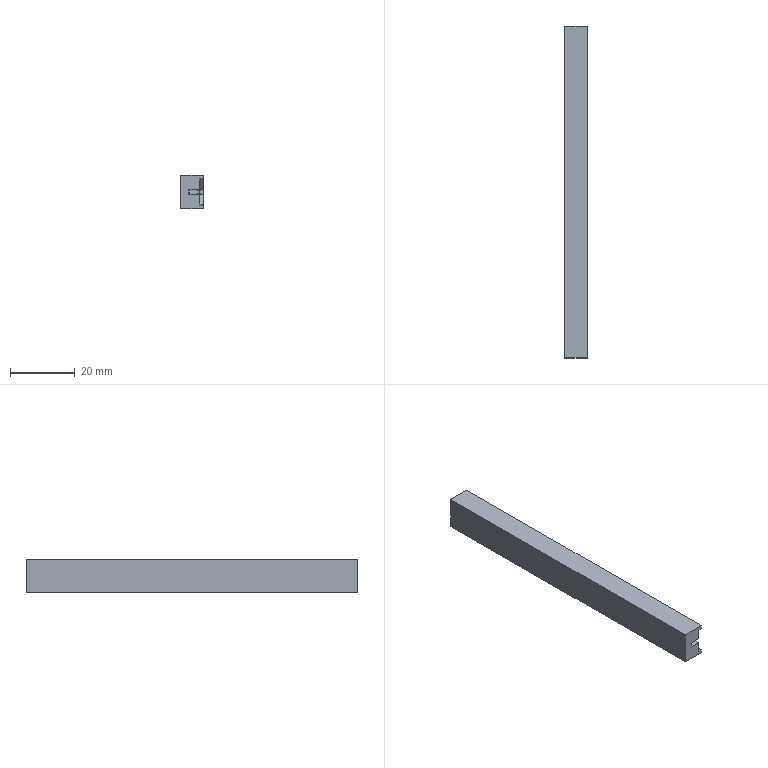Part | STEP file | 1 solid | 17 faces | box 7 x 102.36 x 10.193 mm | volume 7206 mm3 | plane 17
STEP:
#1=CARTESIAN_POINT('',(0.,0.,0.));
#2=DIRECTION('',(0.,0.,1.));
#3=DIRECTION('',(1.,0.,0.));
#4=AXIS2_PLACEMENT_3D('',#1,#2,#3);
#5=CARTESIAN_POINT('',(-126.956,28.14,148.811));
#6=VERTEX_POINT('',#5);
#7=CARTESIAN_POINT('',(-126.956,28.14,147.735));
#8=VERTEX_POINT('',#7);
#9=CARTESIAN_POINT('',(-126.956,28.14,139.695));
#10=DIRECTION('',(0.,0.,-1.));
#11=VECTOR('',#10,1.);
#12=LINE('',#9,#11);
#13=CARTESIAN_POINT('',(-128.063,28.14,139.695));
#14=DIRECTION('',(0.,-1.,0.));
#15=DIRECTION('',(0.,0.,-1.));
#16=AXIS2_PLACEMENT_3D('',#13,#14,#15);
#17=PLANE('',#16);
#18=CARTESIAN_POINT('',(0.,1.107));
#19=DIRECTION('',(1.,0.));
#20=VECTOR('',#19,1.);
#21=LINE('',#18,#20);
#22=(GEOMETRIC_REPRESENTATION_CONTEXT(2)PARAMETRIC_REPRESENTATION_CONTEXT()REPRESENTATION_CONTEXT('',''));
#23=DEFINITIONAL_REPRESENTATION('',(#21),#22);
#24=PCURVE('',#17,#23);
#25=CARTESIAN_POINT('',(-126.956,79.32,143.715));
#26=DIRECTION('',(-1.,0.,0.));
#27=DIRECTION('',(0.,0.,1.));
#28=AXIS2_PLACEMENT_3D('',#25,#26,#27);
#29=PLANE('',#28);
#30=CARTESIAN_POINT('',(-4.02,-51.18));
#31=DIRECTION('',(-1.,0.));
#32=VECTOR('',#31,1.);
#33=LINE('',#30,#32);
#34=(GEOMETRIC_REPRESENTATION_CONTEXT(2)PARAMETRIC_REPRESENTATION_CONTEXT()REPRESENTATION_CONTEXT('',''));
#35=DEFINITIONAL_REPRESENTATION('',(#33),#34);
#36=PCURVE('',#29,#35);
#37=SURFACE_CURVE('',#12,(#24,#36),.PCURVE_S1.);
#38=EDGE_CURVE('',#6,#8,#37,.T.);
#39=ORIENTED_EDGE('',*,*,#38,.F.);
#40=CARTESIAN_POINT('',(-133.956,28.14,148.811));
#41=VERTEX_POINT('',#40);
#42=CARTESIAN_POINT('',(-128.063,28.14,148.811));
#43=DIRECTION('',(-1.,0.,0.));
#44=VECTOR('',#43,1.);
#45=LINE('',#42,#44);
#46=CARTESIAN_POINT('',(-9.117,0.));
#47=DIRECTION('',(0.,-1.));
#48=VECTOR('',#47,1.);
#49=LINE('',#46,#48);
#50=(GEOMETRIC_REPRESENTATION_CONTEXT(2)PARAMETRIC_REPRESENTATION_CONTEXT()REPRESENTATION_CONTEXT('',''));
#51=DEFINITIONAL_REPRESENTATION('',(#49),#50);
#52=PCURVE('',#17,#51);
#53=CARTESIAN_POINT('',(-128.063,32.411,148.811));
#54=DIRECTION('',(0.,0.,1.));
#55=DIRECTION('',(1.,0.,0.));
#56=AXIS2_PLACEMENT_3D('',#53,#54,#55);
#57=PLANE('',#56);
#58=CARTESIAN_POINT('',(0.,-4.271));
#59=DIRECTION('',(-1.,0.));
#60=VECTOR('',#59,1.);
#61=LINE('',#58,#60);
#62=(GEOMETRIC_REPRESENTATION_CONTEXT(2)PARAMETRIC_REPRESENTATION_CONTEXT()REPRESENTATION_CONTEXT('',''));
#63=DEFINITIONAL_REPRESENTATION('',(#61),#62);
#64=PCURVE('',#57,#63);
#65=SURFACE_CURVE('',#45,(#52,#64),.PCURVE_S1.);
#66=EDGE_CURVE('',#6,#41,#65,.T.);
#67=ORIENTED_EDGE('',*,*,#66,.T.);
#68=CARTESIAN_POINT('',(-133.956,28.14,138.619));
#69=VERTEX_POINT('',#68);
#70=CARTESIAN_POINT('',(-133.956,28.14,139.695));
#71=DIRECTION('',(0.,0.,1.));
#72=VECTOR('',#71,1.);
#73=LINE('',#70,#72);
#74=CARTESIAN_POINT('',(0.,-5.893));
#75=DIRECTION('',(-1.,0.));
#76=VECTOR('',#75,1.);
#77=LINE('',#74,#76);
#78=(GEOMETRIC_REPRESENTATION_CONTEXT(2)PARAMETRIC_REPRESENTATION_CONTEXT()REPRESENTATION_CONTEXT('',''));
#79=DEFINITIONAL_REPRESENTATION('',(#77),#78);
#80=PCURVE('',#17,#79);
#81=CARTESIAN_POINT('',(-133.956,32.411,143.715));
#82=DIRECTION('',(1.,0.,0.));
#83=DIRECTION('',(0.,0.,-1.));
#84=AXIS2_PLACEMENT_3D('',#81,#82,#83);
#85=PLANE('',#84);
#86=CARTESIAN_POINT('',(4.02,-4.271));
#87=DIRECTION('',(-1.,0.));
#88=VECTOR('',#87,1.);
#89=LINE('',#86,#88);
#90=(GEOMETRIC_REPRESENTATION_CONTEXT(2)PARAMETRIC_REPRESENTATION_CONTEXT()REPRESENTATION_CONTEXT('',''));
#91=DEFINITIONAL_REPRESENTATION('',(#89),#90);
#92=PCURVE('',#85,#91);
#93=SURFACE_CURVE('',#73,(#80,#92),.PCURVE_S1.);
#94=EDGE_CURVE('',#69,#41,#93,.T.);
#95=ORIENTED_EDGE('',*,*,#94,.F.);
#96=CARTESIAN_POINT('',(-126.956,28.14,138.619));
#97=VERTEX_POINT('',#96);
#98=CARTESIAN_POINT('',(-128.063,28.14,138.619));
#99=DIRECTION('',(1.,0.,0.));
#100=VECTOR('',#99,1.);
#101=LINE('',#98,#100);
#102=CARTESIAN_POINT('',(1.077,0.));
#103=DIRECTION('',(0.,1.));
#104=VECTOR('',#103,1.);
#105=LINE('',#102,#104);
#106=(GEOMETRIC_REPRESENTATION_CONTEXT(2)PARAMETRIC_REPRESENTATION_CONTEXT()REPRESENTATION_CONTEXT('',''));
#107=DEFINITIONAL_REPRESENTATION('',(#105),#106);
#108=PCURVE('',#17,#107);
#109=CARTESIAN_POINT('',(-128.063,32.411,138.619));
#110=DIRECTION('',(0.,0.,-1.));
#111=DIRECTION('',(-1.,0.,0.));
#112=AXIS2_PLACEMENT_3D('',#109,#110,#111);
#113=PLANE('',#112);
#114=CARTESIAN_POINT('',(0.,-4.271));
#115=DIRECTION('',(-1.,0.));
#116=VECTOR('',#115,1.);
#117=LINE('',#114,#116);
#118=(GEOMETRIC_REPRESENTATION_CONTEXT(2)PARAMETRIC_REPRESENTATION_CONTEXT()REPRESENTATION_CONTEXT('',''));
#119=DEFINITIONAL_REPRESENTATION('',(#117),#118);
#120=PCURVE('',#113,#119);
#121=SURFACE_CURVE('',#101,(#108,#120),.PCURVE_S1.);
#122=EDGE_CURVE('',#69,#97,#121,.T.);
#123=ORIENTED_EDGE('',*,*,#122,.T.);
#124=CARTESIAN_POINT('',(-126.956,28.14,139.695));
#125=VERTEX_POINT('',#124);
#126=CARTESIAN_POINT('',(-126.956,28.14,139.695));
#127=DIRECTION('',(0.,0.,-1.));
#128=VECTOR('',#127,1.);
#129=LINE('',#126,#128);
#130=CARTESIAN_POINT('',(0.,1.107));
#131=DIRECTION('',(1.,0.));
#132=VECTOR('',#131,1.);
#133=LINE('',#130,#132);
#134=(GEOMETRIC_REPRESENTATION_CONTEXT(2)PARAMETRIC_REPRESENTATION_CONTEXT()REPRESENTATION_CONTEXT('',''));
#135=DEFINITIONAL_REPRESENTATION('',(#133),#134);
#136=PCURVE('',#17,#135);
#137=CARTESIAN_POINT('',(-4.02,-51.18));
#138=DIRECTION('',(-1.,0.));
#139=VECTOR('',#138,1.);
#140=LINE('',#137,#139);
#141=(GEOMETRIC_REPRESENTATION_CONTEXT(2)PARAMETRIC_REPRESENTATION_CONTEXT()REPRESENTATION_CONTEXT('',''));
#142=DEFINITIONAL_REPRESENTATION('',(#140),#141);
#143=PCURVE('',#29,#142);
#144=SURFACE_CURVE('',#129,(#136,#143),.PCURVE_S1.);
#145=EDGE_CURVE('',#125,#97,#144,.T.);
#146=ORIENTED_EDGE('',*,*,#145,.F.);
#147=CARTESIAN_POINT('',(-128.137,28.14,139.695));
#148=VERTEX_POINT('',#147);
#149=CARTESIAN_POINT('',(-72.862,28.14,139.695));
#150=DIRECTION('',(1.,0.,0.));
#151=VECTOR('',#150,1.);
#152=LINE('',#149,#151);
#153=CARTESIAN_POINT('',(0.,55.2));
#154=DIRECTION('',(0.,1.));
#155=VECTOR('',#154,1.);
#156=LINE('',#153,#155);
#157=(GEOMETRIC_REPRESENTATION_CONTEXT(2)PARAMETRIC_REPRESENTATION_CONTEXT()REPRESENTATION_CONTEXT('',''));
#158=DEFINITIONAL_REPRESENTATION('',(#156),#157);
#159=PCURVE('',#17,#158);
#160=CARTESIAN_POINT('',(-72.862,28.14,139.695));
#161=DIRECTION('',(0.,0.01745,-0.9998));
#162=DIRECTION('',(0.,0.9998,0.01745));
#163=AXIS2_PLACEMENT_3D('',#160,#161,#162);
#164=PLANE('',#163);
#165=CARTESIAN_POINT('',(0.,0.));
#166=DIRECTION('',(0.,1.));
#167=VECTOR('',#166,1.);
#168=LINE('',#165,#167);
#169=(GEOMETRIC_REPRESENTATION_CONTEXT(2)PARAMETRIC_REPRESENTATION_CONTEXT()REPRESENTATION_CONTEXT('',''));
#170=DEFINITIONAL_REPRESENTATION('',(#168),#169);
#171=PCURVE('',#164,#170);
#172=SURFACE_CURVE('',#152,(#159,#171),.PCURVE_S1.);
#173=EDGE_CURVE('',#148,#125,#172,.T.);
#174=ORIENTED_EDGE('',*,*,#173,.F.);
#175=CARTESIAN_POINT('',(-128.137,28.14,142.961));
#176=VERTEX_POINT('',#175);
#177=CARTESIAN_POINT('',(-128.137,28.14,-91.563));
#178=DIRECTION('',(0.,0.,-1.));
#179=VECTOR('',#178,1.);
#180=LINE('',#177,#179);
#181=CARTESIAN_POINT('',(231.258,-0.07455));
#182=DIRECTION('',(1.,0.));
#183=VECTOR('',#182,1.);
#184=LINE('',#181,#183);
#185=(GEOMETRIC_REPRESENTATION_CONTEXT(2)PARAMETRIC_REPRESENTATION_CONTEXT()REPRESENTATION_CONTEXT('',''));
#186=DEFINITIONAL_REPRESENTATION('',(#184),#185);
#187=PCURVE('',#17,#186);
#188=CARTESIAN_POINT('',(-128.137,28.14,-91.563));
#189=DIRECTION('',(-0.9998,0.01745,0.));
#190=DIRECTION('',(-0.01745,-0.9998,0.));
#191=AXIS2_PLACEMENT_3D('',#188,#189,#190);
#192=PLANE('',#191);
#193=CARTESIAN_POINT('',(0.,0.));
#194=DIRECTION('',(0.,-1.));
#195=VECTOR('',#194,1.);
#196=LINE('',#193,#195);
#197=(GEOMETRIC_REPRESENTATION_CONTEXT(2)PARAMETRIC_REPRESENTATION_CONTEXT()REPRESENTATION_CONTEXT('',''));
#198=DEFINITIONAL_REPRESENTATION('',(#196),#197);
#199=PCURVE('',#192,#198);
#200=SURFACE_CURVE('',#180,(#187,#199),.PCURVE_S1.);
#201=EDGE_CURVE('',#176,#148,#200,.T.);
#202=ORIENTED_EDGE('',*,*,#201,.F.);
#203=CARTESIAN_POINT('',(-131.404,28.14,142.961));
#204=VERTEX_POINT('',#203);
#205=CARTESIAN_POINT('',(-72.862,28.14,142.961));
#206=DIRECTION('',(-1.,0.,0.));
#207=VECTOR('',#206,1.);
#208=LINE('',#205,#207);
#209=CARTESIAN_POINT('',(-3.266,55.2));
#210=DIRECTION('',(0.,-1.));
#211=VECTOR('',#210,1.);
#212=LINE('',#209,#211);
#213=(GEOMETRIC_REPRESENTATION_CONTEXT(2)PARAMETRIC_REPRESENTATION_CONTEXT()REPRESENTATION_CONTEXT('',''));
#214=DEFINITIONAL_REPRESENTATION('',(#212),#213);
#215=PCURVE('',#17,#214);
#216=CARTESIAN_POINT('',(-72.862,28.14,142.961));
#217=DIRECTION('',(0.,0.01745,-0.9998));
#218=DIRECTION('',(0.,0.9998,0.01745));
#219=AXIS2_PLACEMENT_3D('',#216,#217,#218);
#220=PLANE('',#219);
#221=CARTESIAN_POINT('',(0.,0.));
#222=DIRECTION('',(0.,-1.));
#223=VECTOR('',#222,1.);
#224=LINE('',#221,#223);
#225=(GEOMETRIC_REPRESENTATION_CONTEXT(2)PARAMETRIC_REPRESENTATION_CONTEXT()REPRESENTATION_CONTEXT('',''));
#226=DEFINITIONAL_REPRESENTATION('',(#224),#225);
#227=PCURVE('',#220,#226);
#228=SURFACE_CURVE('',#208,(#215,#227),.PCURVE_S1.);
#229=EDGE_CURVE('',#176,#204,#228,.T.);
#230=ORIENTED_EDGE('',*,*,#229,.T.);
#231=CARTESIAN_POINT('',(-131.404,28.14,144.469));
#232=VERTEX_POINT('',#231);
#233=CARTESIAN_POINT('',(-131.404,28.14,-91.563));
#234=DIRECTION('',(0.,0.,-1.));
#235=VECTOR('',#234,1.);
#236=LINE('',#233,#235);
#237=CARTESIAN_POINT('',(231.258,-3.341));
#238=DIRECTION('',(1.,0.));
#239=VECTOR('',#238,1.);
#240=LINE('',#237,#239);
#241=(GEOMETRIC_REPRESENTATION_CONTEXT(2)PARAMETRIC_REPRESENTATION_CONTEXT()REPRESENTATION_CONTEXT('',''));
#242=DEFINITIONAL_REPRESENTATION('',(#240),#241);
#243=PCURVE('',#17,#242);
#244=CARTESIAN_POINT('',(-131.404,28.14,-91.563));
#245=DIRECTION('',(-0.9998,0.01745,0.));
#246=DIRECTION('',(-0.01745,-0.9998,0.));
#247=AXIS2_PLACEMENT_3D('',#244,#245,#246);
#248=PLANE('',#247);
#249=CARTESIAN_POINT('',(0.,0.));
#250=DIRECTION('',(0.,-1.));
#251=VECTOR('',#250,1.);
#252=LINE('',#249,#251);
#253=(GEOMETRIC_REPRESENTATION_CONTEXT(2)PARAMETRIC_REPRESENTATION_CONTEXT()REPRESENTATION_CONTEXT('',''));
#254=DEFINITIONAL_REPRESENTATION('',(#252),#253);
#255=PCURVE('',#248,#254);
#256=SURFACE_CURVE('',#236,(#243,#255),.PCURVE_S1.);
#257=EDGE_CURVE('',#232,#204,#256,.T.);
#258=ORIENTED_EDGE('',*,*,#257,.F.);
#259=CARTESIAN_POINT('',(-128.137,28.14,144.469));
#260=VERTEX_POINT('',#259);
#261=CARTESIAN_POINT('',(-72.862,28.14,144.469));
#262=DIRECTION('',(-1.,0.,0.));
#263=VECTOR('',#262,1.);
#264=LINE('',#261,#263);
#265=CARTESIAN_POINT('',(-4.774,55.2));
#266=DIRECTION('',(0.,-1.));
#267=VECTOR('',#266,1.);
#268=LINE('',#265,#267);
#269=(GEOMETRIC_REPRESENTATION_CONTEXT(2)PARAMETRIC_REPRESENTATION_CONTEXT()REPRESENTATION_CONTEXT('',''));
#270=DEFINITIONAL_REPRESENTATION('',(#268),#269);
#271=PCURVE('',#17,#270);
#272=CARTESIAN_POINT('',(-72.862,28.14,144.469));
#273=DIRECTION('',(0.,0.01745,0.9998));
#274=DIRECTION('',(0.,-0.9998,0.01745));
#275=AXIS2_PLACEMENT_3D('',#272,#273,#274);
#276=PLANE('',#275);
#277=CARTESIAN_POINT('',(0.,0.));
#278=DIRECTION('',(0.,-1.));
#279=VECTOR('',#278,1.);
#280=LINE('',#277,#279);
#281=(GEOMETRIC_REPRESENTATION_CONTEXT(2)PARAMETRIC_REPRESENTATION_CONTEXT()REPRESENTATION_CONTEXT('',''));
#282=DEFINITIONAL_REPRESENTATION('',(#280),#281);
#283=PCURVE('',#276,#282);
#284=SURFACE_CURVE('',#264,(#271,#283),.PCURVE_S1.);
#285=EDGE_CURVE('',#260,#232,#284,.T.);
#286=ORIENTED_EDGE('',*,*,#285,.F.);
#287=CARTESIAN_POINT('',(-128.137,28.14,147.735));
#288=VERTEX_POINT('',#287);
#289=CARTESIAN_POINT('',(-128.137,28.14,-91.563));
#290=DIRECTION('',(0.,0.,-1.));
#291=VECTOR('',#290,1.);
#292=LINE('',#289,#291);
#293=CARTESIAN_POINT('',(231.258,-0.07455));
#294=DIRECTION('',(1.,0.));
#295=VECTOR('',#294,1.);
#296=LINE('',#293,#295);
#297=(GEOMETRIC_REPRESENTATION_CONTEXT(2)PARAMETRIC_REPRESENTATION_CONTEXT()REPRESENTATION_CONTEXT('',''));
#298=DEFINITIONAL_REPRESENTATION('',(#296),#297);
#299=PCURVE('',#17,#298);
#300=CARTESIAN_POINT('',(-128.137,28.14,-91.563));
#301=DIRECTION('',(-0.9998,0.01745,0.));
#302=DIRECTION('',(-0.01745,-0.9998,0.));
#303=AXIS2_PLACEMENT_3D('',#300,#301,#302);
#304=PLANE('',#303);
#305=CARTESIAN_POINT('',(0.,0.));
#306=DIRECTION('',(0.,-1.));
#307=VECTOR('',#306,1.);
#308=LINE('',#305,#307);
#309=(GEOMETRIC_REPRESENTATION_CONTEXT(2)PARAMETRIC_REPRESENTATION_CONTEXT()REPRESENTATION_CONTEXT('',''));
#310=DEFINITIONAL_REPRESENTATION('',(#308),#309);
#311=PCURVE('',#304,#310);
#312=SURFACE_CURVE('',#292,(#299,#311),.PCURVE_S1.);
#313=EDGE_CURVE('',#288,#260,#312,.T.);
#314=ORIENTED_EDGE('',*,*,#313,.F.);
#315=CARTESIAN_POINT('',(-72.862,28.14,147.735));
#316=DIRECTION('',(-1.,0.,0.));
#317=VECTOR('',#316,1.);
#318=LINE('',#315,#317);
#319=CARTESIAN_POINT('',(-8.04,55.2));
#320=DIRECTION('',(0.,-1.));
#321=VECTOR('',#320,1.);
#322=LINE('',#319,#321);
#323=(GEOMETRIC_REPRESENTATION_CONTEXT(2)PARAMETRIC_REPRESENTATION_CONTEXT()REPRESENTATION_CONTEXT('',''));
#324=DEFINITIONAL_REPRESENTATION('',(#322),#323);
#325=PCURVE('',#17,#324);
#326=CARTESIAN_POINT('',(-72.862,28.14,147.735));
#327=DIRECTION('',(0.,0.01745,0.9998));
#328=DIRECTION('',(0.,-0.9998,0.01745));
#329=AXIS2_PLACEMENT_3D('',#326,#327,#328);
#330=PLANE('',#329);
#331=CARTESIAN_POINT('',(0.,0.));
#332=DIRECTION('',(0.,-1.));
#333=VECTOR('',#332,1.);
#334=LINE('',#331,#333);
#335=(GEOMETRIC_REPRESENTATION_CONTEXT(2)PARAMETRIC_REPRESENTATION_CONTEXT()REPRESENTATION_CONTEXT('',''));
#336=DEFINITIONAL_REPRESENTATION('',(#334),#335);
#337=PCURVE('',#330,#336);
#338=SURFACE_CURVE('',#318,(#325,#337),.PCURVE_S1.);
#339=EDGE_CURVE('',#8,#288,#338,.T.);
#340=ORIENTED_EDGE('',*,*,#339,.F.);
#341=EDGE_LOOP('',(#39,#67,#95,#123,#146,#174,#202,#230,#258,#286,#314,#340));
#342=FACE_BOUND('',#341,.T.);
#343=ADVANCED_FACE('',(#342),#17,.T.);
#344=CARTESIAN_POINT('',(-126.956,130.5,148.811));
#345=VERTEX_POINT('',#344);
#346=CARTESIAN_POINT('',(-126.956,32.411,148.811));
#347=DIRECTION('',(0.,-1.,0.));
#348=VECTOR('',#347,1.);
#349=LINE('',#346,#348);
#350=CARTESIAN_POINT('',(1.107,0.));
#351=DIRECTION('',(0.,-1.));
#352=VECTOR('',#351,1.);
#353=LINE('',#350,#352);
#354=(GEOMETRIC_REPRESENTATION_CONTEXT(2)PARAMETRIC_REPRESENTATION_CONTEXT()REPRESENTATION_CONTEXT('',''));
#355=DEFINITIONAL_REPRESENTATION('',(#353),#354);
#356=PCURVE('',#57,#355);
#357=CARTESIAN_POINT('',(5.096,-46.909));
#358=DIRECTION('',(0.,-1.));
#359=VECTOR('',#358,1.);
#360=LINE('',#357,#359);
#361=(GEOMETRIC_REPRESENTATION_CONTEXT(2)PARAMETRIC_REPRESENTATION_CONTEXT()REPRESENTATION_CONTEXT('',''));
#362=DEFINITIONAL_REPRESENTATION('',(#360),#361);
#363=PCURVE('',#29,#362);
#364=SURFACE_CURVE('',#349,(#356,#363),.PCURVE_S1.);
#365=EDGE_CURVE('',#345,#6,#364,.T.);
#366=ORIENTED_EDGE('',*,*,#365,.F.);
#367=CARTESIAN_POINT('',(-133.956,130.5,148.811));
#368=VERTEX_POINT('',#367);
#369=CARTESIAN_POINT('',(-72.862,130.5,148.811));
#370=DIRECTION('',(1.,0.,0.));
#371=VECTOR('',#370,1.);
#372=LINE('',#369,#371);
#373=CARTESIAN_POINT('',(55.2,98.089));
#374=DIRECTION('',(1.,0.));
#375=VECTOR('',#374,1.);
#376=LINE('',#373,#375);
#377=(GEOMETRIC_REPRESENTATION_CONTEXT(2)PARAMETRIC_REPRESENTATION_CONTEXT()REPRESENTATION_CONTEXT('',''));
#378=DEFINITIONAL_REPRESENTATION('',(#376),#377);
#379=PCURVE('',#57,#378);
#380=CARTESIAN_POINT('',(-72.862,130.5,110.196));
#381=DIRECTION('',(0.,-1.,0.));
#382=DIRECTION('',(0.,0.,-1.));
#383=AXIS2_PLACEMENT_3D('',#380,#381,#382);
#384=PLANE('',#383);
#385=CARTESIAN_POINT('',(-38.616,0.));
#386=DIRECTION('',(0.,1.));
#387=VECTOR('',#386,1.);
#388=LINE('',#385,#387);
#389=(GEOMETRIC_REPRESENTATION_CONTEXT(2)PARAMETRIC_REPRESENTATION_CONTEXT()REPRESENTATION_CONTEXT('',''));
#390=DEFINITIONAL_REPRESENTATION('',(#388),#389);
#391=PCURVE('',#384,#390);
#392=SURFACE_CURVE('',#372,(#379,#391),.PCURVE_S1.);
#393=EDGE_CURVE('',#368,#345,#392,.T.);
#394=ORIENTED_EDGE('',*,*,#393,.F.);
#395=CARTESIAN_POINT('',(-133.956,32.411,148.811));
#396=DIRECTION('',(0.,1.,0.));
#397=VECTOR('',#396,1.);
#398=LINE('',#395,#397);
#399=CARTESIAN_POINT('',(-5.893,0.));
#400=DIRECTION('',(0.,1.));
#401=VECTOR('',#400,1.);
#402=LINE('',#399,#401);
#403=(GEOMETRIC_REPRESENTATION_CONTEXT(2)PARAMETRIC_REPRESENTATION_CONTEXT()REPRESENTATION_CONTEXT('',''));
#404=DEFINITIONAL_REPRESENTATION('',(#402),#403);
#405=PCURVE('',#57,#404);
#406=CARTESIAN_POINT('',(-5.096,0.));
#407=DIRECTION('',(0.,1.));
#408=VECTOR('',#407,1.);
#409=LINE('',#406,#408);
#410=(GEOMETRIC_REPRESENTATION_CONTEXT(2)PARAMETRIC_REPRESENTATION_CONTEXT()REPRESENTATION_CONTEXT('',''));
#411=DEFINITIONAL_REPRESENTATION('',(#409),#410);
#412=PCURVE('',#85,#411);
#413=SURFACE_CURVE('',#398,(#405,#412),.PCURVE_S1.);
#414=EDGE_CURVE('',#41,#368,#413,.T.);
#415=ORIENTED_EDGE('',*,*,#414,.F.);
#416=ORIENTED_EDGE('',*,*,#66,.F.);
#417=EDGE_LOOP('',(#366,#394,#415,#416));
#418=FACE_BOUND('',#417,.T.);
#419=ADVANCED_FACE('',(#418),#57,.T.);
#420=CARTESIAN_POINT('',(-126.956,130.5,138.619));
#421=VERTEX_POINT('',#420);
#422=CARTESIAN_POINT('',(-126.956,130.5,110.196));
#423=DIRECTION('',(0.,0.,1.));
#424=VECTOR('',#423,1.);
#425=LINE('',#422,#424);
#426=CARTESIAN_POINT('',(0.,-54.094));
#427=DIRECTION('',(-1.,0.));
#428=VECTOR('',#427,1.);
#429=LINE('',#426,#428);
#430=(GEOMETRIC_REPRESENTATION_CONTEXT(2)PARAMETRIC_REPRESENTATION_CONTEXT()REPRESENTATION_CONTEXT('',''));
#431=DEFINITIONAL_REPRESENTATION('',(#429),#430);
#432=PCURVE('',#384,#431);
#433=CARTESIAN_POINT('',(-33.519,51.18));
#434=DIRECTION('',(1.,0.));
#435=VECTOR('',#434,1.);
#436=LINE('',#433,#435);
#437=(GEOMETRIC_REPRESENTATION_CONTEXT(2)PARAMETRIC_REPRESENTATION_CONTEXT()REPRESENTATION_CONTEXT('',''));
#438=DEFINITIONAL_REPRESENTATION('',(#436),#437);
#439=PCURVE('',#29,#438);
#440=SURFACE_CURVE('',#425,(#432,#439),.PCURVE_S1.);
#441=EDGE_CURVE('',#421,#345,#440,.T.);
#442=ORIENTED_EDGE('',*,*,#441,.F.);
#443=CARTESIAN_POINT('',(-133.956,130.5,138.619));
#444=VERTEX_POINT('',#443);
#445=CARTESIAN_POINT('',(-72.862,130.5,138.619));
#446=DIRECTION('',(-1.,0.,0.));
#447=VECTOR('',#446,1.);
#448=LINE('',#445,#447);
#449=CARTESIAN_POINT('',(-28.423,0.));
#450=DIRECTION('',(0.,-1.));
#451=VECTOR('',#450,1.);
#452=LINE('',#449,#451);
#453=(GEOMETRIC_REPRESENTATION_CONTEXT(2)PARAMETRIC_REPRESENTATION_CONTEXT()REPRESENTATION_CONTEXT('',''));
#454=DEFINITIONAL_REPRESENTATION('',(#452),#453);
#455=PCURVE('',#384,#454);
#456=CARTESIAN_POINT('',(-55.2,98.089));
#457=DIRECTION('',(1.,0.));
#458=VECTOR('',#457,1.);
#459=LINE('',#456,#458);
#460=(GEOMETRIC_REPRESENTATION_CONTEXT(2)PARAMETRIC_REPRESENTATION_CONTEXT()REPRESENTATION_CONTEXT('',''));
#461=DEFINITIONAL_REPRESENTATION('',(#459),#460);
#462=PCURVE('',#113,#461);
#463=SURFACE_CURVE('',#448,(#455,#462),.PCURVE_S1.);
#464=EDGE_CURVE('',#421,#444,#463,.T.);
#465=ORIENTED_EDGE('',*,*,#464,.T.);
#466=CARTESIAN_POINT('',(-133.956,130.5,110.196));
#467=DIRECTION('',(0.,0.,-1.));
#468=VECTOR('',#467,1.);
#469=LINE('',#466,#468);
#470=CARTESIAN_POINT('',(0.,-61.094));
#471=DIRECTION('',(1.,0.));
#472=VECTOR('',#471,1.);
#473=LINE('',#470,#472);
#474=(GEOMETRIC_REPRESENTATION_CONTEXT(2)PARAMETRIC_REPRESENTATION_CONTEXT()REPRESENTATION_CONTEXT('',''));
#475=DEFINITIONAL_REPRESENTATION('',(#473),#474);
#476=PCURVE('',#384,#475);
#477=CARTESIAN_POINT('',(33.519,98.089));
#478=DIRECTION('',(1.,0.));
#479=VECTOR('',#478,1.);
#480=LINE('',#477,#479);
#481=(GEOMETRIC_REPRESENTATION_CONTEXT(2)PARAMETRIC_REPRESENTATION_CONTEXT()REPRESENTATION_CONTEXT('',''));
#482=DEFINITIONAL_REPRESENTATION('',(#480),#481);
#483=PCURVE('',#85,#482);
#484=SURFACE_CURVE('',#469,(#476,#483),.PCURVE_S1.);
#485=EDGE_CURVE('',#368,#444,#484,.T.);
#486=ORIENTED_EDGE('',*,*,#485,.F.);
#487=ORIENTED_EDGE('',*,*,#393,.T.);
#488=EDGE_LOOP('',(#442,#465,#486,#487));
#489=FACE_BOUND('',#488,.T.);
#490=ADVANCED_FACE('',(#489),#384,.F.);
#491=CARTESIAN_POINT('',(-126.956,32.411,138.619));
#492=DIRECTION('',(0.,1.,0.));
#493=VECTOR('',#492,1.);
#494=LINE('',#491,#493);
#495=CARTESIAN_POINT('',(-1.107,0.));
#496=DIRECTION('',(0.,1.));
#497=VECTOR('',#496,1.);
#498=LINE('',#495,#497);
#499=(GEOMETRIC_REPRESENTATION_CONTEXT(2)PARAMETRIC_REPRESENTATION_CONTEXT()REPRESENTATION_CONTEXT('',''));
#500=DEFINITIONAL_REPRESENTATION('',(#498),#499);
#501=PCURVE('',#113,#500);
#502=CARTESIAN_POINT('',(-5.096,-46.909));
#503=DIRECTION('',(0.,1.));
#504=VECTOR('',#503,1.);
#505=LINE('',#502,#504);
#506=(GEOMETRIC_REPRESENTATION_CONTEXT(2)PARAMETRIC_REPRESENTATION_CONTEXT()REPRESENTATION_CONTEXT('',''));
#507=DEFINITIONAL_REPRESENTATION('',(#505),#506);
#508=PCURVE('',#29,#507);
#509=SURFACE_CURVE('',#494,(#501,#508),.PCURVE_S1.);
#510=EDGE_CURVE('',#97,#421,#509,.T.);
#511=ORIENTED_EDGE('',*,*,#510,.F.);
#512=ORIENTED_EDGE('',*,*,#122,.F.);
#513=CARTESIAN_POINT('',(-133.956,32.411,138.619));
#514=DIRECTION('',(0.,-1.,0.));
#515=VECTOR('',#514,1.);
#516=LINE('',#513,#515);
#517=CARTESIAN_POINT('',(5.893,0.));
#518=DIRECTION('',(0.,-1.));
#519=VECTOR('',#518,1.);
#520=LINE('',#517,#519);
#521=(GEOMETRIC_REPRESENTATION_CONTEXT(2)PARAMETRIC_REPRESENTATION_CONTEXT()REPRESENTATION_CONTEXT('',''));
#522=DEFINITIONAL_REPRESENTATION('',(#520),#521);
#523=PCURVE('',#113,#522);
#524=CARTESIAN_POINT('',(5.096,0.));
#525=DIRECTION('',(0.,-1.));
#526=VECTOR('',#525,1.);
#527=LINE('',#524,#526);
#528=(GEOMETRIC_REPRESENTATION_CONTEXT(2)PARAMETRIC_REPRESENTATION_CONTEXT()REPRESENTATION_CONTEXT('',''));
#529=DEFINITIONAL_REPRESENTATION('',(#527),#528);
#530=PCURVE('',#85,#529);
#531=SURFACE_CURVE('',#516,(#523,#530),.PCURVE_S1.);
#532=EDGE_CURVE('',#444,#69,#531,.T.);
#533=ORIENTED_EDGE('',*,*,#532,.F.);
#534=ORIENTED_EDGE('',*,*,#464,.F.);
#535=EDGE_LOOP('',(#511,#512,#533,#534));
#536=FACE_BOUND('',#535,.T.);
#537=ADVANCED_FACE('',(#536),#113,.T.);
#538=ORIENTED_EDGE('',*,*,#414,.T.);
#539=ORIENTED_EDGE('',*,*,#485,.T.);
#540=ORIENTED_EDGE('',*,*,#532,.T.);
#541=ORIENTED_EDGE('',*,*,#94,.T.);
#542=EDGE_LOOP('',(#538,#539,#540,#541));
#543=FACE_BOUND('',#542,.T.);
#544=ADVANCED_FACE('',(#543),#85,.F.);
#545=CARTESIAN_POINT('',(-128.186,36.682,144.32));
#546=VERTEX_POINT('',#545);
#547=CARTESIAN_POINT('',(-131.307,33.668,144.372));
#548=VERTEX_POINT('',#547);
#549=CARTESIAN_POINT('',(-103.832,60.2,143.909));
#550=DIRECTION('',(-0.7193,-0.6946,0.01212));
#551=VECTOR('',#550,1.);
#552=LINE('',#549,#551);
#553=CARTESIAN_POINT('',(-131.307,33.668,-91.563));
#554=DIRECTION('',(0.6947,-0.7193,0.));
#555=DIRECTION('',(0.7193,0.6947,0.));
#556=AXIS2_PLACEMENT_3D('',#553,#554,#555);
#557=PLANE('',#556);
#558=CARTESIAN_POINT('',(38.195,235.472));
#559=DIRECTION('',(-0.9999,0.01212));
#560=VECTOR('',#559,1.);
#561=LINE('',#558,#560);
#562=(GEOMETRIC_REPRESENTATION_CONTEXT(2)PARAMETRIC_REPRESENTATION_CONTEXT()REPRESENTATION_CONTEXT('',''));
#563=DEFINITIONAL_REPRESENTATION('',(#561),#562);
#564=PCURVE('',#557,#563);
#565=CARTESIAN_POINT('',(-32.065,-30.97));
#566=DIRECTION('',(0.6947,-0.7193));
#567=VECTOR('',#566,1.);
#568=LINE('',#565,#567);
#569=(GEOMETRIC_REPRESENTATION_CONTEXT(2)PARAMETRIC_REPRESENTATION_CONTEXT()REPRESENTATION_CONTEXT('',''));
#570=DEFINITIONAL_REPRESENTATION('',(#568),#569);
#571=PCURVE('',#276,#570);
#572=SURFACE_CURVE('',#552,(#564,#571),.PCURVE_S1.);
#573=EDGE_CURVE('',#546,#548,#572,.T.);
#574=ORIENTED_EDGE('',*,*,#573,.T.);
#575=CARTESIAN_POINT('',(-131.307,33.668,143.058));
#576=VERTEX_POINT('',#575);
#577=CARTESIAN_POINT('',(-131.307,33.668,-91.563));
#578=DIRECTION('',(0.,0.,-1.));
#579=VECTOR('',#578,1.);
#580=LINE('',#577,#579);
#581=CARTESIAN_POINT('',(0.,0.));
#582=DIRECTION('',(0.,-1.));
#583=VECTOR('',#582,1.);
#584=LINE('',#581,#583);
#585=(GEOMETRIC_REPRESENTATION_CONTEXT(2)PARAMETRIC_REPRESENTATION_CONTEXT()REPRESENTATION_CONTEXT('',''));
#586=DEFINITIONAL_REPRESENTATION('',(#584),#585);
#587=PCURVE('',#557,#586);
#588=CARTESIAN_POINT('',(-5.529,0.));
#589=DIRECTION('',(0.,-1.));
#590=VECTOR('',#589,1.);
#591=LINE('',#588,#590);
#592=(GEOMETRIC_REPRESENTATION_CONTEXT(2)PARAMETRIC_REPRESENTATION_CONTEXT()REPRESENTATION_CONTEXT('',''));
#593=DEFINITIONAL_REPRESENTATION('',(#591),#592);
#594=PCURVE('',#248,#593);
#595=SURFACE_CURVE('',#580,(#587,#594),.PCURVE_S1.);
#596=EDGE_CURVE('',#548,#576,#595,.T.);
#597=ORIENTED_EDGE('',*,*,#596,.T.);
#598=CARTESIAN_POINT('',(-128.186,36.682,143.11));
#599=VERTEX_POINT('',#598);
#600=CARTESIAN_POINT('',(-133.353,31.692,143.023));
#601=DIRECTION('',(0.7193,0.6946,0.01212));
#602=VECTOR('',#601,1.);
#603=LINE('',#600,#602);
#604=CARTESIAN_POINT('',(-2.844,234.587));
#605=DIRECTION('',(0.9999,0.01212));
#606=VECTOR('',#605,1.);
#607=LINE('',#604,#606);
#608=(GEOMETRIC_REPRESENTATION_CONTEXT(2)PARAMETRIC_REPRESENTATION_CONTEXT()REPRESENTATION_CONTEXT('',''));
#609=DEFINITIONAL_REPRESENTATION('',(#607),#608);
#610=PCURVE('',#557,#609);
#611=CARTESIAN_POINT('',(3.553,-60.491));
#612=DIRECTION('',(0.6947,0.7193));
#613=VECTOR('',#612,1.);
#614=LINE('',#611,#613);
#615=(GEOMETRIC_REPRESENTATION_CONTEXT(2)PARAMETRIC_REPRESENTATION_CONTEXT()REPRESENTATION_CONTEXT('',''));
#616=DEFINITIONAL_REPRESENTATION('',(#614),#615);
#617=PCURVE('',#220,#616);
#618=SURFACE_CURVE('',#603,(#610,#617),.PCURVE_S1.);
#619=EDGE_CURVE('',#576,#599,#618,.T.);
#620=ORIENTED_EDGE('',*,*,#619,.T.);
#621=CARTESIAN_POINT('',(-128.186,36.682,144.469));
#622=DIRECTION('',(0.,0.,1.));
#623=VECTOR('',#622,1.);
#624=LINE('',#621,#623);
#625=CARTESIAN_POINT('',(4.34,236.032));
#626=DIRECTION('',(0.,1.));
#627=VECTOR('',#626,1.);
#628=LINE('',#625,#627);
#629=(GEOMETRIC_REPRESENTATION_CONTEXT(2)PARAMETRIC_REPRESENTATION_CONTEXT()REPRESENTATION_CONTEXT('',''));
#630=DEFINITIONAL_REPRESENTATION('',(#628),#629);
#631=PCURVE('',#557,#630);
#632=CARTESIAN_POINT('',(-131.404,36.682,144.469));
#633=DIRECTION('',(0.,1.,0.));
#634=DIRECTION('',(0.,0.,1.));
#635=AXIS2_PLACEMENT_3D('',#632,#633,#634);
#636=PLANE('',#635);
#637=CARTESIAN_POINT('',(0.,3.218));
#638=DIRECTION('',(1.,0.));
#639=VECTOR('',#638,1.);
#640=LINE('',#637,#639);
#641=(GEOMETRIC_REPRESENTATION_CONTEXT(2)PARAMETRIC_REPRESENTATION_CONTEXT()REPRESENTATION_CONTEXT('',''));
#642=DEFINITIONAL_REPRESENTATION('',(#640),#641);
#643=PCURVE('',#636,#642);
#644=SURFACE_CURVE('',#624,(#631,#643),.PCURVE_S1.);
#645=EDGE_CURVE('',#599,#546,#644,.T.);
#646=ORIENTED_EDGE('',*,*,#645,.T.);
#647=EDGE_LOOP('',(#574,#597,#620,#646));
#648=FACE_BOUND('',#647,.T.);
#649=ADVANCED_FACE('',(#648),#557,.T.);
#650=CARTESIAN_POINT('',(-128.041,33.668,139.791));
#651=VERTEX_POINT('',#650);
#652=CARTESIAN_POINT('',(-126.956,33.668,139.791));
#653=VERTEX_POINT('',#652);
#654=CARTESIAN_POINT('',(-72.862,33.668,139.791));
#655=DIRECTION('',(1.,0.,0.));
#656=VECTOR('',#655,1.);
#657=LINE('',#654,#656);
#658=CARTESIAN_POINT('',(-72.862,33.668,139.791));
#659=DIRECTION('',(0.,-0.7193,0.6947));
#660=DIRECTION('',(0.,-0.6947,-0.7193));
#661=AXIS2_PLACEMENT_3D('',#658,#659,#660);
#662=PLANE('',#661);
#663=CARTESIAN_POINT('',(0.,0.));
#664=DIRECTION('',(0.,1.));
#665=VECTOR('',#664,1.);
#666=LINE('',#663,#665);
#667=(GEOMETRIC_REPRESENTATION_CONTEXT(2)PARAMETRIC_REPRESENTATION_CONTEXT()REPRESENTATION_CONTEXT('',''));
#668=DEFINITIONAL_REPRESENTATION('',(#666),#667);
#669=PCURVE('',#662,#668);
#670=CARTESIAN_POINT('',(5.529,0.));
#671=DIRECTION('',(0.,1.));
#672=VECTOR('',#671,1.);
#673=LINE('',#670,#672);
#674=(GEOMETRIC_REPRESENTATION_CONTEXT(2)PARAMETRIC_REPRESENTATION_CONTEXT()REPRESENTATION_CONTEXT('',''));
#675=DEFINITIONAL_REPRESENTATION('',(#673),#674);
#676=PCURVE('',#164,#675);
#677=SURFACE_CURVE('',#657,(#669,#676),.PCURVE_S1.);
#678=EDGE_CURVE('',#651,#653,#677,.T.);
#679=ORIENTED_EDGE('',*,*,#678,.T.);
#680=CARTESIAN_POINT('',(-126.956,36.682,142.913));
#681=VERTEX_POINT('',#680);
#682=CARTESIAN_POINT('',(-126.956,33.668,139.791));
#683=DIRECTION('',(0.,0.6947,0.7193));
#684=VECTOR('',#683,1.);
#685=LINE('',#682,#684);
#686=CARTESIAN_POINT('',(0.,-54.094));
#687=DIRECTION('',(-1.,0.));
#688=VECTOR('',#687,1.);
#689=LINE('',#686,#688);
#690=(GEOMETRIC_REPRESENTATION_CONTEXT(2)PARAMETRIC_REPRESENTATION_CONTEXT()REPRESENTATION_CONTEXT('',''));
#691=DEFINITIONAL_REPRESENTATION('',(#689),#690);
#692=PCURVE('',#662,#691);
#693=CARTESIAN_POINT('',(-3.924,-45.652));
#694=DIRECTION('',(0.7193,0.6947));
#695=VECTOR('',#694,1.);
#696=LINE('',#693,#695);
#697=(GEOMETRIC_REPRESENTATION_CONTEXT(2)PARAMETRIC_REPRESENTATION_CONTEXT()REPRESENTATION_CONTEXT('',''));
#698=DEFINITIONAL_REPRESENTATION('',(#696),#697);
#699=PCURVE('',#29,#698);
#700=SURFACE_CURVE('',#685,(#692,#699),.PCURVE_S1.);
#701=EDGE_CURVE('',#653,#681,#700,.T.);
#702=ORIENTED_EDGE('',*,*,#701,.T.);
#703=CARTESIAN_POINT('',(-127.988,36.682,142.913));
#704=VERTEX_POINT('',#703);
#705=CARTESIAN_POINT('',(-131.404,36.682,142.913));
#706=DIRECTION('',(-1.,0.,0.));
#707=VECTOR('',#706,1.);
#708=LINE('',#705,#707);
#709=CARTESIAN_POINT('',(-4.34,-58.541));
#710=DIRECTION('',(0.,-1.));
#711=VECTOR('',#710,1.);
#712=LINE('',#709,#711);
#713=(GEOMETRIC_REPRESENTATION_CONTEXT(2)PARAMETRIC_REPRESENTATION_CONTEXT()REPRESENTATION_CONTEXT('',''));
#714=DEFINITIONAL_REPRESENTATION('',(#712),#713);
#715=PCURVE('',#662,#714);
#716=CARTESIAN_POINT('',(-1.556,0.));
#717=DIRECTION('',(0.,-1.));
#718=VECTOR('',#717,1.);
#719=LINE('',#716,#718);
#720=(GEOMETRIC_REPRESENTATION_CONTEXT(2)PARAMETRIC_REPRESENTATION_CONTEXT()REPRESENTATION_CONTEXT('',''));
#721=DEFINITIONAL_REPRESENTATION('',(#719),#720);
#722=PCURVE('',#636,#721);
#723=SURFACE_CURVE('',#708,(#715,#722),.PCURVE_S1.);
#724=EDGE_CURVE('',#681,#704,#723,.T.);
#725=ORIENTED_EDGE('',*,*,#724,.T.);
#726=CARTESIAN_POINT('',(-130.105,-84.59,17.332));
#727=DIRECTION('',(-0.01212,-0.6946,-0.7193));
#728=VECTOR('',#727,1.);
#729=LINE('',#726,#728);
#730=CARTESIAN_POINT('',(170.239,-57.243));
#731=DIRECTION('',(0.9999,-0.01212));
#732=VECTOR('',#731,1.);
#733=LINE('',#730,#732);
#734=(GEOMETRIC_REPRESENTATION_CONTEXT(2)PARAMETRIC_REPRESENTATION_CONTEXT()REPRESENTATION_CONTEXT('',''));
#735=DEFINITIONAL_REPRESENTATION('',(#733),#734);
#736=PCURVE('',#662,#735);
#737=CARTESIAN_POINT('',(112.747,108.895));
#738=DIRECTION('',(0.6947,-0.7193));
#739=VECTOR('',#738,1.);
#740=LINE('',#737,#739);
#741=(GEOMETRIC_REPRESENTATION_CONTEXT(2)PARAMETRIC_REPRESENTATION_CONTEXT()REPRESENTATION_CONTEXT('',''));
#742=DEFINITIONAL_REPRESENTATION('',(#740),#741);
#743=PCURVE('',#192,#742);
#744=SURFACE_CURVE('',#729,(#736,#743),.PCURVE_S1.);
#745=EDGE_CURVE('',#704,#651,#744,.T.);
#746=ORIENTED_EDGE('',*,*,#745,.T.);
#747=EDGE_LOOP('',(#679,#702,#725,#746));
#748=FACE_BOUND('',#747,.T.);
#749=ADVANCED_FACE('',(#748),#662,.T.);
#750=ORIENTED_EDGE('',*,*,#724,.F.);
#751=CARTESIAN_POINT('',(-126.956,36.682,144.517));
#752=VERTEX_POINT('',#751);
#753=CARTESIAN_POINT('',(-126.956,36.682,144.469));
#754=DIRECTION('',(0.,0.,1.));
#755=VECTOR('',#754,1.);
#756=LINE('',#753,#755);
#757=CARTESIAN_POINT('',(0.,4.447));
#758=DIRECTION('',(1.,0.));
#759=VECTOR('',#758,1.);
#760=LINE('',#757,#759);
#761=(GEOMETRIC_REPRESENTATION_CONTEXT(2)PARAMETRIC_REPRESENTATION_CONTEXT()REPRESENTATION_CONTEXT('',''));
#762=DEFINITIONAL_REPRESENTATION('',(#760),#761);
#763=PCURVE('',#636,#762);
#764=CARTESIAN_POINT('',(0.7538,-42.638));
#765=DIRECTION('',(1.,0.));
#766=VECTOR('',#765,1.);
#767=LINE('',#764,#766);
#768=(GEOMETRIC_REPRESENTATION_CONTEXT(2)PARAMETRIC_REPRESENTATION_CONTEXT()REPRESENTATION_CONTEXT('',''));
#769=DEFINITIONAL_REPRESENTATION('',(#767),#768);
#770=PCURVE('',#29,#769);
#771=SURFACE_CURVE('',#756,(#763,#770),.PCURVE_S1.);
#772=EDGE_CURVE('',#681,#752,#771,.T.);
#773=ORIENTED_EDGE('',*,*,#772,.T.);
#774=CARTESIAN_POINT('',(-127.988,36.682,144.517));
#775=VERTEX_POINT('',#774);
#776=CARTESIAN_POINT('',(-131.404,36.682,144.517));
#777=DIRECTION('',(1.,0.,0.));
#778=VECTOR('',#777,1.);
#779=LINE('',#776,#778);
#780=CARTESIAN_POINT('',(0.04811,0.));
#781=DIRECTION('',(0.,1.));
#782=VECTOR('',#781,1.);
#783=LINE('',#780,#782);
#784=(GEOMETRIC_REPRESENTATION_CONTEXT(2)PARAMETRIC_REPRESENTATION_CONTEXT()REPRESENTATION_CONTEXT('',''));
#785=DEFINITIONAL_REPRESENTATION('',(#783),#784);
#786=PCURVE('',#636,#785);
#787=CARTESIAN_POINT('',(-72.862,33.668,147.639));
#788=DIRECTION('',(0.,-0.7193,-0.6947));
#789=DIRECTION('',(0.,0.6947,-0.7193));
#790=AXIS2_PLACEMENT_3D('',#787,#788,#789);
#791=PLANE('',#790);
#792=CARTESIAN_POINT('',(4.34,-58.541));
#793=DIRECTION('',(0.,1.));
#794=VECTOR('',#793,1.);
#795=LINE('',#792,#794);
#796=(GEOMETRIC_REPRESENTATION_CONTEXT(2)PARAMETRIC_REPRESENTATION_CONTEXT()REPRESENTATION_CONTEXT('',''));
#797=DEFINITIONAL_REPRESENTATION('',(#795),#796);
#798=PCURVE('',#791,#797);
#799=SURFACE_CURVE('',#779,(#786,#798),.PCURVE_S1.);
#800=EDGE_CURVE('',#775,#752,#799,.T.);
#801=ORIENTED_EDGE('',*,*,#800,.F.);
#802=CARTESIAN_POINT('',(-127.988,36.682,144.32));
#803=VERTEX_POINT('',#802);
#804=CARTESIAN_POINT('',(-127.988,36.682,-91.563));
#805=DIRECTION('',(0.,0.,-1.));
#806=VECTOR('',#805,1.);
#807=LINE('',#804,#806);
#808=CARTESIAN_POINT('',(-236.032,3.415));
#809=DIRECTION('',(-1.,0.));
#810=VECTOR('',#809,1.);
#811=LINE('',#808,#810);
#812=(GEOMETRIC_REPRESENTATION_CONTEXT(2)PARAMETRIC_REPRESENTATION_CONTEXT()REPRESENTATION_CONTEXT('',''));
#813=DEFINITIONAL_REPRESENTATION('',(#811),#812);
#814=PCURVE('',#636,#813);
#815=CARTESIAN_POINT('',(-8.544,0.));
#816=DIRECTION('',(0.,-1.));
#817=VECTOR('',#816,1.);
#818=LINE('',#815,#817);
#819=(GEOMETRIC_REPRESENTATION_CONTEXT(2)PARAMETRIC_REPRESENTATION_CONTEXT()REPRESENTATION_CONTEXT('',''));
#820=DEFINITIONAL_REPRESENTATION('',(#818),#819);
#821=PCURVE('',#304,#820);
#822=SURFACE_CURVE('',#807,(#814,#821),.PCURVE_S1.);
#823=EDGE_CURVE('',#775,#803,#822,.T.);
#824=ORIENTED_EDGE('',*,*,#823,.T.);
#825=CARTESIAN_POINT('',(-131.404,36.682,144.32));
#826=DIRECTION('',(1.,0.,0.));
#827=VECTOR('',#826,1.);
#828=LINE('',#825,#827);
#829=CARTESIAN_POINT('',(-0.1491,0.));
#830=DIRECTION('',(0.,1.));
#831=VECTOR('',#830,1.);
#832=LINE('',#829,#831);
#833=(GEOMETRIC_REPRESENTATION_CONTEXT(2)PARAMETRIC_REPRESENTATION_CONTEXT()REPRESENTATION_CONTEXT('',''));
#834=DEFINITIONAL_REPRESENTATION('',(#832),#833);
#835=PCURVE('',#636,#834);
#836=CARTESIAN_POINT('',(-8.544,-58.541));
#837=DIRECTION('',(0.,1.));
#838=VECTOR('',#837,1.);
#839=LINE('',#836,#838);
#840=(GEOMETRIC_REPRESENTATION_CONTEXT(2)PARAMETRIC_REPRESENTATION_CONTEXT()REPRESENTATION_CONTEXT('',''));
#841=DEFINITIONAL_REPRESENTATION('',(#839),#840);
#842=PCURVE('',#276,#841);
#843=SURFACE_CURVE('',#828,(#835,#842),.PCURVE_S1.);
#844=EDGE_CURVE('',#546,#803,#843,.T.);
#845=ORIENTED_EDGE('',*,*,#844,.F.);
#846=ORIENTED_EDGE('',*,*,#645,.F.);
#847=CARTESIAN_POINT('',(-127.988,36.682,143.11));
#848=VERTEX_POINT('',#847);
#849=CARTESIAN_POINT('',(-131.404,36.682,143.11));
#850=DIRECTION('',(1.,0.,0.));
#851=VECTOR('',#850,1.);
#852=LINE('',#849,#851);
#853=CARTESIAN_POINT('',(-1.358,0.));
#854=DIRECTION('',(0.,1.));
#855=VECTOR('',#854,1.);
#856=LINE('',#853,#855);
#857=(GEOMETRIC_REPRESENTATION_CONTEXT(2)PARAMETRIC_REPRESENTATION_CONTEXT()REPRESENTATION_CONTEXT('',''));
#858=DEFINITIONAL_REPRESENTATION('',(#856),#857);
#859=PCURVE('',#636,#858);
#860=CARTESIAN_POINT('',(8.544,-58.541));
#861=DIRECTION('',(0.,1.));
#862=VECTOR('',#861,1.);
#863=LINE('',#860,#862);
#864=(GEOMETRIC_REPRESENTATION_CONTEXT(2)PARAMETRIC_REPRESENTATION_CONTEXT()REPRESENTATION_CONTEXT('',''));
#865=DEFINITIONAL_REPRESENTATION('',(#863),#864);
#866=PCURVE('',#220,#865);
#867=SURFACE_CURVE('',#852,(#859,#866),.PCURVE_S1.);
#868=EDGE_CURVE('',#599,#848,#867,.T.);
#869=ORIENTED_EDGE('',*,*,#868,.T.);
#870=CARTESIAN_POINT('',(-127.988,36.682,-91.563));
#871=DIRECTION('',(0.,0.,-1.));
#872=VECTOR('',#871,1.);
#873=LINE('',#870,#872);
#874=CARTESIAN_POINT('',(-236.032,3.415));
#875=DIRECTION('',(-1.,0.));
#876=VECTOR('',#875,1.);
#877=LINE('',#874,#876);
#878=(GEOMETRIC_REPRESENTATION_CONTEXT(2)PARAMETRIC_REPRESENTATION_CONTEXT()REPRESENTATION_CONTEXT('',''));
#879=DEFINITIONAL_REPRESENTATION('',(#877),#878);
#880=PCURVE('',#636,#879);
#881=CARTESIAN_POINT('',(-8.544,0.));
#882=DIRECTION('',(0.,-1.));
#883=VECTOR('',#882,1.);
#884=LINE('',#881,#883);
#885=(GEOMETRIC_REPRESENTATION_CONTEXT(2)PARAMETRIC_REPRESENTATION_CONTEXT()REPRESENTATION_CONTEXT('',''));
#886=DEFINITIONAL_REPRESENTATION('',(#884),#885);
#887=PCURVE('',#192,#886);
#888=SURFACE_CURVE('',#873,(#880,#887),.PCURVE_S1.);
#889=EDGE_CURVE('',#848,#704,#888,.T.);
#890=ORIENTED_EDGE('',*,*,#889,.T.);
#891=EDGE_LOOP('',(#750,#773,#801,#824,#845,#846,#869,#890));
#892=FACE_BOUND('',#891,.T.);
#893=ADVANCED_FACE('',(#892),#636,.F.);
#894=ORIENTED_EDGE('',*,*,#800,.T.);
#895=CARTESIAN_POINT('',(-126.956,33.668,147.639));
#896=VERTEX_POINT('',#895);
#897=CARTESIAN_POINT('',(-126.956,33.668,147.639));
#898=DIRECTION('',(0.,-0.6947,0.7193));
#899=VECTOR('',#898,1.);
#900=LINE('',#897,#899);
#901=CARTESIAN_POINT('',(0.,-54.094));
#902=DIRECTION('',(-1.,0.));
#903=VECTOR('',#902,1.);
#904=LINE('',#901,#903);
#905=(GEOMETRIC_REPRESENTATION_CONTEXT(2)PARAMETRIC_REPRESENTATION_CONTEXT()REPRESENTATION_CONTEXT('',''));
#906=DEFINITIONAL_REPRESENTATION('',(#904),#905);
#907=PCURVE('',#791,#906);
#908=CARTESIAN_POINT('',(3.924,-45.652));
#909=DIRECTION('',(0.7193,-0.6947));
#910=VECTOR('',#909,1.);
#911=LINE('',#908,#910);
#912=(GEOMETRIC_REPRESENTATION_CONTEXT(2)PARAMETRIC_REPRESENTATION_CONTEXT()REPRESENTATION_CONTEXT('',''));
#913=DEFINITIONAL_REPRESENTATION('',(#911),#912);
#914=PCURVE('',#29,#913);
#915=SURFACE_CURVE('',#900,(#907,#914),.PCURVE_S1.);
#916=EDGE_CURVE('',#752,#896,#915,.T.);
#917=ORIENTED_EDGE('',*,*,#916,.T.);
#918=CARTESIAN_POINT('',(-128.041,33.668,147.639));
#919=VERTEX_POINT('',#918);
#920=CARTESIAN_POINT('',(-72.862,33.668,147.639));
#921=DIRECTION('',(-1.,0.,0.));
#922=VECTOR('',#921,1.);
#923=LINE('',#920,#922);
#924=CARTESIAN_POINT('',(0.,0.));
#925=DIRECTION('',(0.,-1.));
#926=VECTOR('',#925,1.);
#927=LINE('',#924,#926);
#928=(GEOMETRIC_REPRESENTATION_CONTEXT(2)PARAMETRIC_REPRESENTATION_CONTEXT()REPRESENTATION_CONTEXT('',''));
#929=DEFINITIONAL_REPRESENTATION('',(#927),#928);
#930=PCURVE('',#791,#929);
#931=CARTESIAN_POINT('',(-5.529,0.));
#932=DIRECTION('',(0.,-1.));
#933=VECTOR('',#932,1.);
#934=LINE('',#931,#933);
#935=(GEOMETRIC_REPRESENTATION_CONTEXT(2)PARAMETRIC_REPRESENTATION_CONTEXT()REPRESENTATION_CONTEXT('',''));
#936=DEFINITIONAL_REPRESENTATION('',(#934),#935);
#937=PCURVE('',#330,#936);
#938=SURFACE_CURVE('',#923,(#930,#937),.PCURVE_S1.);
#939=EDGE_CURVE('',#896,#919,#938,.T.);
#940=ORIENTED_EDGE('',*,*,#939,.T.);
#941=CARTESIAN_POINT('',(-126.002,150.511,26.645));
#942=DIRECTION('',(0.01212,0.6946,-0.7193));
#943=VECTOR('',#942,1.);
#944=LINE('',#941,#943);
#945=CARTESIAN_POINT('',(168.201,-53.139));
#946=DIRECTION('',(0.9999,0.01212));
#947=VECTOR('',#946,1.);
#948=LINE('',#945,#947);
#949=(GEOMETRIC_REPRESENTATION_CONTEXT(2)PARAMETRIC_REPRESENTATION_CONTEXT()REPRESENTATION_CONTEXT('',''));
#950=DEFINITIONAL_REPRESENTATION('',(#948),#949);
#951=PCURVE('',#791,#950);
#952=CARTESIAN_POINT('',(-122.389,118.208));
#953=DIRECTION('',(-0.6947,-0.7193));
#954=VECTOR('',#953,1.);
#955=LINE('',#952,#954);
#956=(GEOMETRIC_REPRESENTATION_CONTEXT(2)PARAMETRIC_REPRESENTATION_CONTEXT()REPRESENTATION_CONTEXT('',''));
#957=DEFINITIONAL_REPRESENTATION('',(#955),#956);
#958=PCURVE('',#304,#957);
#959=SURFACE_CURVE('',#944,(#951,#958),.PCURVE_S1.);
#960=EDGE_CURVE('',#919,#775,#959,.T.);
#961=ORIENTED_EDGE('',*,*,#960,.T.);
#962=EDGE_LOOP('',(#894,#917,#940,#961));
#963=FACE_BOUND('',#962,.T.);
#964=ADVANCED_FACE('',(#963),#791,.T.);
#965=CARTESIAN_POINT('',(-128.121,29.104,147.718));
#966=DIRECTION('',(-0.01745,-0.9997,0.01745));
#967=VECTOR('',#966,1.);
#968=LINE('',#965,#967);
#969=CARTESIAN_POINT('',(-0.9644,239.282));
#970=DIRECTION('',(0.9998,0.01745));
#971=VECTOR('',#970,1.);
#972=LINE('',#969,#971);
#973=(GEOMETRIC_REPRESENTATION_CONTEXT(2)PARAMETRIC_REPRESENTATION_CONTEXT()REPRESENTATION_CONTEXT('',''));
#974=DEFINITIONAL_REPRESENTATION('',(#972),#973);
#975=PCURVE('',#304,#974);
#976=CARTESIAN_POINT('',(-0.9644,-55.258));
#977=DIRECTION('',(0.9998,-0.01745));
#978=VECTOR('',#977,1.);
#979=LINE('',#976,#978);
#980=(GEOMETRIC_REPRESENTATION_CONTEXT(2)PARAMETRIC_REPRESENTATION_CONTEXT()REPRESENTATION_CONTEXT('',''));
#981=DEFINITIONAL_REPRESENTATION('',(#979),#980);
#982=PCURVE('',#330,#981);
#983=SURFACE_CURVE('',#968,(#975,#982),.PCURVE_S1.);
#984=EDGE_CURVE('',#919,#288,#983,.T.);
#985=ORIENTED_EDGE('',*,*,#984,.T.);
#986=ORIENTED_EDGE('',*,*,#313,.T.);
#987=CARTESIAN_POINT('',(-128.121,29.104,144.452));
#988=DIRECTION('',(-0.01745,-0.9997,0.01745));
#989=VECTOR('',#988,1.);
#990=LINE('',#987,#989);
#991=CARTESIAN_POINT('',(-0.9644,236.015));
#992=DIRECTION('',(0.9998,0.01745));
#993=VECTOR('',#992,1.);
#994=LINE('',#991,#993);
#995=(GEOMETRIC_REPRESENTATION_CONTEXT(2)PARAMETRIC_REPRESENTATION_CONTEXT()REPRESENTATION_CONTEXT('',''));
#996=DEFINITIONAL_REPRESENTATION('',(#994),#995);
#997=PCURVE('',#304,#996);
#998=CARTESIAN_POINT('',(-0.9644,-55.258));
#999=DIRECTION('',(0.9998,-0.01745));
#1000=VECTOR('',#999,1.);
#1001=LINE('',#998,#1000);
#1002=(GEOMETRIC_REPRESENTATION_CONTEXT(2)PARAMETRIC_REPRESENTATION_CONTEXT()REPRESENTATION_CONTEXT('',''));
#1003=DEFINITIONAL_REPRESENTATION('',(#1001),#1002);
#1004=PCURVE('',#276,#1003);
#1005=SURFACE_CURVE('',#990,(#997,#1004),.PCURVE_S1.);
#1006=EDGE_CURVE('',#803,#260,#1005,.T.);
#1007=ORIENTED_EDGE('',*,*,#1006,.F.);
#1008=ORIENTED_EDGE('',*,*,#823,.F.);
#1009=ORIENTED_EDGE('',*,*,#960,.F.);
#1010=EDGE_LOOP('',(#985,#986,#1007,#1008,#1009));
#1011=FACE_BOUND('',#1010,.T.);
#1012=ADVANCED_FACE('',(#1011),#304,.F.);
#1013=ORIENTED_EDGE('',*,*,#844,.T.);
#1014=ORIENTED_EDGE('',*,*,#1006,.T.);
#1015=ORIENTED_EDGE('',*,*,#285,.T.);
#1016=CARTESIAN_POINT('',(-131.332,32.257,144.397));
#1017=DIRECTION('',(0.01745,0.9997,-0.01745));
#1018=VECTOR('',#1017,1.);
#1019=LINE('',#1016,#1018);
#1020=CARTESIAN_POINT('',(-4.118,-58.469));
#1021=DIRECTION('',(-0.9998,0.01745));
#1022=VECTOR('',#1021,1.);
#1023=LINE('',#1020,#1022);
#1024=(GEOMETRIC_REPRESENTATION_CONTEXT(2)PARAMETRIC_REPRESENTATION_CONTEXT()REPRESENTATION_CONTEXT('',''));
#1025=DEFINITIONAL_REPRESENTATION('',(#1023),#1024);
#1026=PCURVE('',#276,#1025);
#1027=CARTESIAN_POINT('',(-4.118,235.96));
#1028=DIRECTION('',(-0.9998,-0.01745));
#1029=VECTOR('',#1028,1.);
#1030=LINE('',#1027,#1029);
#1031=(GEOMETRIC_REPRESENTATION_CONTEXT(2)PARAMETRIC_REPRESENTATION_CONTEXT()REPRESENTATION_CONTEXT('',''));
#1032=DEFINITIONAL_REPRESENTATION('',(#1030),#1031);
#1033=PCURVE('',#248,#1032);
#1034=SURFACE_CURVE('',#1019,(#1026,#1033),.PCURVE_S1.);
#1035=EDGE_CURVE('',#232,#548,#1034,.T.);
#1036=ORIENTED_EDGE('',*,*,#1035,.T.);
#1037=ORIENTED_EDGE('',*,*,#573,.F.);
#1038=EDGE_LOOP('',(#1013,#1014,#1015,#1036,#1037));
#1039=FACE_BOUND('',#1038,.T.);
#1040=ADVANCED_FACE('',(#1039),#276,.F.);
#1041=ORIENTED_EDGE('',*,*,#1035,.F.);
#1042=ORIENTED_EDGE('',*,*,#257,.T.);
#1043=CARTESIAN_POINT('',(-131.475,24.049,142.89));
#1044=DIRECTION('',(0.01745,0.9997,0.01745));
#1045=VECTOR('',#1044,1.);
#1046=LINE('',#1043,#1045);
#1047=CARTESIAN_POINT('',(4.092,234.453));
#1048=DIRECTION('',(-0.9998,0.01745));
#1049=VECTOR('',#1048,1.);
#1050=LINE('',#1047,#1049);
#1051=(GEOMETRIC_REPRESENTATION_CONTEXT(2)PARAMETRIC_REPRESENTATION_CONTEXT()REPRESENTATION_CONTEXT('',''));
#1052=DEFINITIONAL_REPRESENTATION('',(#1050),#1051);
#1053=PCURVE('',#248,#1052);
#1054=CARTESIAN_POINT('',(-4.092,-58.613));
#1055=DIRECTION('',(0.9998,0.01745));
#1056=VECTOR('',#1055,1.);
#1057=LINE('',#1054,#1056);
#1058=(GEOMETRIC_REPRESENTATION_CONTEXT(2)PARAMETRIC_REPRESENTATION_CONTEXT()REPRESENTATION_CONTEXT('',''));
#1059=DEFINITIONAL_REPRESENTATION('',(#1057),#1058);
#1060=PCURVE('',#220,#1059);
#1061=SURFACE_CURVE('',#1046,(#1053,#1060),.PCURVE_S1.);
#1062=EDGE_CURVE('',#204,#576,#1061,.T.);
#1063=ORIENTED_EDGE('',*,*,#1062,.T.);
#1064=ORIENTED_EDGE('',*,*,#596,.F.);
#1065=EDGE_LOOP('',(#1041,#1042,#1063,#1064));
#1066=FACE_BOUND('',#1065,.T.);
#1067=ADVANCED_FACE('',(#1066),#248,.F.);
#1068=ORIENTED_EDGE('',*,*,#1062,.F.);
#1069=ORIENTED_EDGE('',*,*,#229,.F.);
#1070=CARTESIAN_POINT('',(-128.121,29.104,142.978));
#1071=DIRECTION('',(-0.01745,-0.9997,-0.01745));
#1072=VECTOR('',#1071,1.);
#1073=LINE('',#1070,#1072);
#1074=CARTESIAN_POINT('',(0.9644,-55.258));
#1075=DIRECTION('',(-0.9998,-0.01745));
#1076=VECTOR('',#1075,1.);
#1077=LINE('',#1074,#1076);
#1078=(GEOMETRIC_REPRESENTATION_CONTEXT(2)PARAMETRIC_REPRESENTATION_CONTEXT()REPRESENTATION_CONTEXT('',''));
#1079=DEFINITIONAL_REPRESENTATION('',(#1077),#1078);
#1080=PCURVE('',#220,#1079);
#1081=CARTESIAN_POINT('',(-0.9644,234.541));
#1082=DIRECTION('',(0.9998,-0.01745));
#1083=VECTOR('',#1082,1.);
#1084=LINE('',#1081,#1083);
#1085=(GEOMETRIC_REPRESENTATION_CONTEXT(2)PARAMETRIC_REPRESENTATION_CONTEXT()REPRESENTATION_CONTEXT('',''));
#1086=DEFINITIONAL_REPRESENTATION('',(#1084),#1085);
#1087=PCURVE('',#192,#1086);
#1088=SURFACE_CURVE('',#1073,(#1080,#1087),.PCURVE_S1.);
#1089=EDGE_CURVE('',#848,#176,#1088,.T.);
#1090=ORIENTED_EDGE('',*,*,#1089,.F.);
#1091=ORIENTED_EDGE('',*,*,#868,.F.);
#1092=ORIENTED_EDGE('',*,*,#619,.F.);
#1093=EDGE_LOOP('',(#1068,#1069,#1090,#1091,#1092));
#1094=FACE_BOUND('',#1093,.T.);
#1095=ADVANCED_FACE('',(#1094),#220,.F.);
#1096=ORIENTED_EDGE('',*,*,#889,.F.);
#1097=ORIENTED_EDGE('',*,*,#1089,.T.);
#1098=ORIENTED_EDGE('',*,*,#201,.T.);
#1099=CARTESIAN_POINT('',(-128.208,24.106,139.625));
#1100=DIRECTION('',(-0.01745,-0.9997,-0.01745));
#1101=VECTOR('',#1100,1.);
#1102=LINE('',#1099,#1101);
#1103=CARTESIAN_POINT('',(4.035,231.188));
#1104=DIRECTION('',(0.9998,-0.01745));
#1105=VECTOR('',#1104,1.);
#1106=LINE('',#1103,#1105);
#1107=(GEOMETRIC_REPRESENTATION_CONTEXT(2)PARAMETRIC_REPRESENTATION_CONTEXT()REPRESENTATION_CONTEXT('',''));
#1108=DEFINITIONAL_REPRESENTATION('',(#1106),#1107);
#1109=PCURVE('',#192,#1108);
#1110=CARTESIAN_POINT('',(-4.035,-55.345));
#1111=DIRECTION('',(-0.9998,-0.01745));
#1112=VECTOR('',#1111,1.);
#1113=LINE('',#1110,#1112);
#1114=(GEOMETRIC_REPRESENTATION_CONTEXT(2)PARAMETRIC_REPRESENTATION_CONTEXT()REPRESENTATION_CONTEXT('',''));
#1115=DEFINITIONAL_REPRESENTATION('',(#1113),#1114);
#1116=PCURVE('',#164,#1115);
#1117=SURFACE_CURVE('',#1102,(#1109,#1116),.PCURVE_S1.);
#1118=EDGE_CURVE('',#651,#148,#1117,.T.);
#1119=ORIENTED_EDGE('',*,*,#1118,.F.);
#1120=ORIENTED_EDGE('',*,*,#745,.F.);
#1121=EDGE_LOOP('',(#1096,#1097,#1098,#1119,#1120));
#1122=FACE_BOUND('',#1121,.T.);
#1123=ADVANCED_FACE('',(#1122),#192,.F.);
#1124=ORIENTED_EDGE('',*,*,#173,.T.);
#1125=CARTESIAN_POINT('',(-126.956,28.14,139.695));
#1126=DIRECTION('',(0.,0.9998,0.01745));
#1127=VECTOR('',#1126,1.);
#1128=LINE('',#1125,#1127);
#1129=CARTESIAN_POINT('',(0.,-54.094));
#1130=DIRECTION('',(1.,0.));
#1131=VECTOR('',#1130,1.);
#1132=LINE('',#1129,#1131);
#1133=(GEOMETRIC_REPRESENTATION_CONTEXT(2)PARAMETRIC_REPRESENTATION_CONTEXT()REPRESENTATION_CONTEXT('',''));
#1134=DEFINITIONAL_REPRESENTATION('',(#1132),#1133);
#1135=PCURVE('',#164,#1134);
#1136=CARTESIAN_POINT('',(-4.02,-51.18));
#1137=DIRECTION('',(0.01745,0.9998));
#1138=VECTOR('',#1137,1.);
#1139=LINE('',#1136,#1138);
#1140=(GEOMETRIC_REPRESENTATION_CONTEXT(2)PARAMETRIC_REPRESENTATION_CONTEXT()REPRESENTATION_CONTEXT('',''));
#1141=DEFINITIONAL_REPRESENTATION('',(#1139),#1140);
#1142=PCURVE('',#29,#1141);
#1143=SURFACE_CURVE('',#1128,(#1135,#1142),.PCURVE_S1.);
#1144=EDGE_CURVE('',#125,#653,#1143,.T.);
#1145=ORIENTED_EDGE('',*,*,#1144,.T.);
#1146=ORIENTED_EDGE('',*,*,#678,.F.);
#1147=ORIENTED_EDGE('',*,*,#1118,.T.);
#1148=EDGE_LOOP('',(#1124,#1145,#1146,#1147));
#1149=FACE_BOUND('',#1148,.T.);
#1150=ADVANCED_FACE('',(#1149),#164,.F.);
#1151=ORIENTED_EDGE('',*,*,#939,.F.);
#1152=CARTESIAN_POINT('',(-126.956,28.14,147.735));
#1153=DIRECTION('',(0.,-0.9998,0.01745));
#1154=VECTOR('',#1153,1.);
#1155=LINE('',#1152,#1154);
#1156=CARTESIAN_POINT('',(0.,-54.094));
#1157=DIRECTION('',(1.,0.));
#1158=VECTOR('',#1157,1.);
#1159=LINE('',#1156,#1158);
#1160=(GEOMETRIC_REPRESENTATION_CONTEXT(2)PARAMETRIC_REPRESENTATION_CONTEXT()REPRESENTATION_CONTEXT('',''));
#1161=DEFINITIONAL_REPRESENTATION('',(#1159),#1160);
#1162=PCURVE('',#330,#1161);
#1163=CARTESIAN_POINT('',(4.02,-51.18));
#1164=DIRECTION('',(0.01745,-0.9998));
#1165=VECTOR('',#1164,1.);
#1166=LINE('',#1163,#1165);
#1167=(GEOMETRIC_REPRESENTATION_CONTEXT(2)PARAMETRIC_REPRESENTATION_CONTEXT()REPRESENTATION_CONTEXT('',''));
#1168=DEFINITIONAL_REPRESENTATION('',(#1166),#1167);
#1169=PCURVE('',#29,#1168);
#1170=SURFACE_CURVE('',#1155,(#1162,#1169),.PCURVE_S1.);
#1171=EDGE_CURVE('',#896,#8,#1170,.T.);
#1172=ORIENTED_EDGE('',*,*,#1171,.T.);
#1173=ORIENTED_EDGE('',*,*,#339,.T.);
#1174=ORIENTED_EDGE('',*,*,#984,.F.);
#1175=EDGE_LOOP('',(#1151,#1172,#1173,#1174));
#1176=FACE_BOUND('',#1175,.T.);
#1177=ADVANCED_FACE('',(#1176),#330,.F.);
#1178=ORIENTED_EDGE('',*,*,#441,.T.);
#1179=ORIENTED_EDGE('',*,*,#365,.T.);
#1180=ORIENTED_EDGE('',*,*,#38,.T.);
#1181=ORIENTED_EDGE('',*,*,#1171,.F.);
#1182=ORIENTED_EDGE('',*,*,#916,.F.);
#1183=ORIENTED_EDGE('',*,*,#772,.F.);
#1184=ORIENTED_EDGE('',*,*,#701,.F.);
#1185=ORIENTED_EDGE('',*,*,#1144,.F.);
#1186=ORIENTED_EDGE('',*,*,#145,.T.);
#1187=ORIENTED_EDGE('',*,*,#510,.T.);
#1188=EDGE_LOOP('',(#1178,#1179,#1180,#1181,#1182,#1183,#1184,#1185,#1186,#1187));
#1189=FACE_BOUND('',#1188,.T.);
#1190=ADVANCED_FACE('',(#1189),#29,.F.);
#1191=CLOSED_SHELL('',(#343,#419,#490,#537,#544,#649,#749,#893,#964,#1012,#1040,#1067,#1095,#1123,#1150,#1177,#1190));
#1192=MANIFOLD_SOLID_BREP('',#1191);
#1193=(LENGTH_UNIT()NAMED_UNIT(*)SI_UNIT(.MILLI.,.METRE.));
#1194=UNCERTAINTY_MEASURE_WITH_UNIT(LENGTH_MEASURE(0.0000001),#1193,'','');
#1195=(NAMED_UNIT(*)PLANE_ANGLE_UNIT()SI_UNIT($,.RADIAN.));
#1196=(NAMED_UNIT(*)SI_UNIT($,.STERADIAN.)SOLID_ANGLE_UNIT());
#1197=(GEOMETRIC_REPRESENTATION_CONTEXT(3)GLOBAL_UNCERTAINTY_ASSIGNED_CONTEXT((#1194))GLOBAL_UNIT_ASSIGNED_CONTEXT((#1193,#1195,#1196))REPRESENTATION_CONTEXT('',''));
#1198=ADVANCED_BREP_SHAPE_REPRESENTATION('',(#4,#1192),#1197);